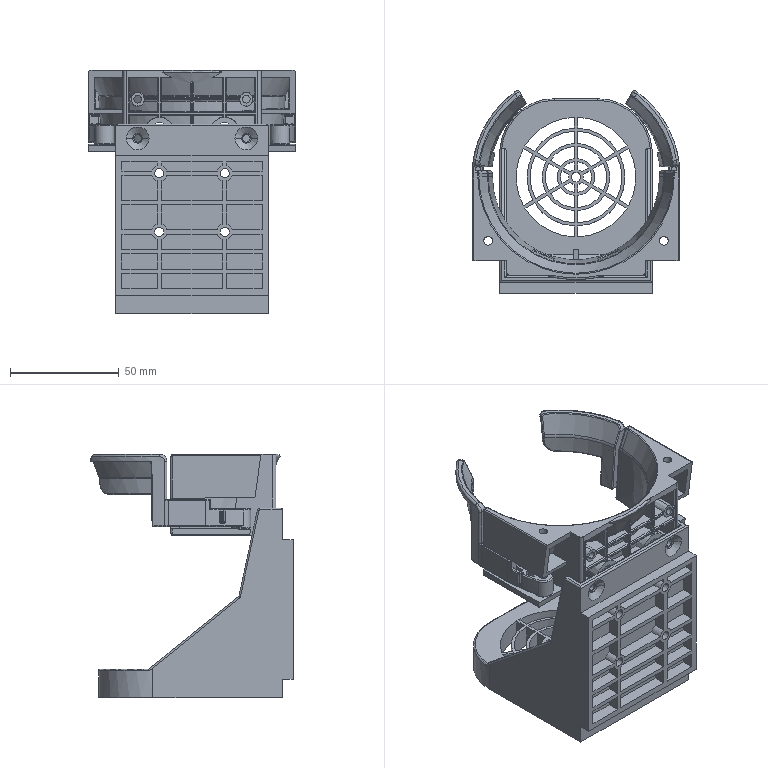Part | SolidWorks | features MBimport 1 | 4 solids | 1024 faces | box 95.114 x 93.076 x 111.7 mm | volume 101033 mm3 | plane 384 | cylinder 284 | cone 147 | torus 99 | spline 94 | sphere 16 | commonest cylinder face diameters 1 x108 4 x21 7.2 x16 1.5 x15 4.2 x10 2 x8